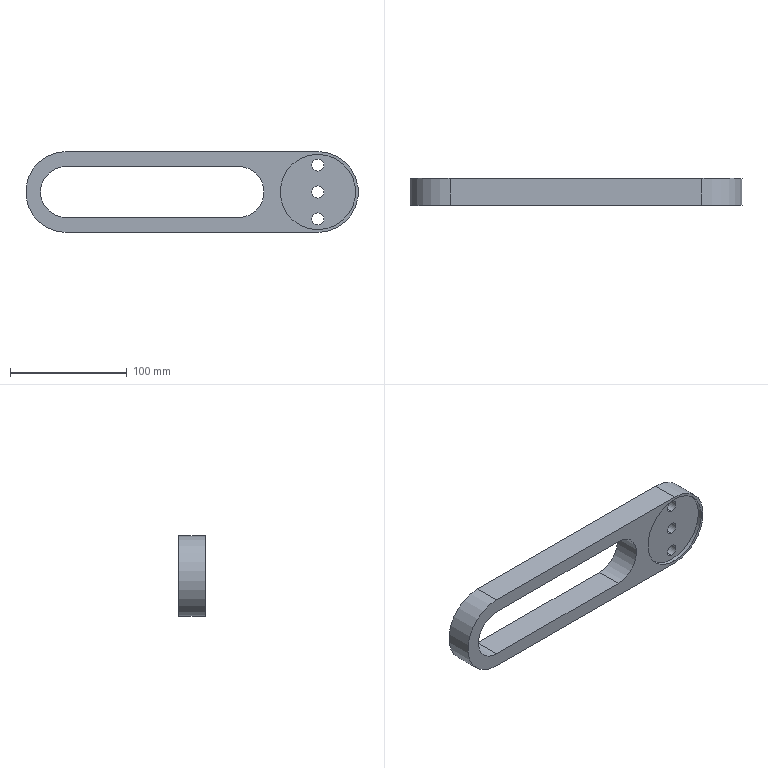Part | SolidWorks | features BaseBody 1 | 1 solid | 28 faces | box 285 x 23.077 x 69.231 mm | volume 225142 mm3 | cylinder 18 | plane 10 | commonest cylinder face diameters 10.385 x6 18.462 x6 43.846 x2 64.615 x2 69.231 x2
STEP:
#1=CARTESIAN_POINT('',(207.247,318.5,260.));
#2=VERTEX_POINT('',#1);
#3=CARTESIAN_POINT('',(207.247,318.5,278.462));
#4=VERTEX_POINT('',#3);
#5=CARTESIAN_POINT('',(207.247,318.5,269.231));
#6=DIRECTION('',(0.,1.,0.));
#7=DIRECTION('',(0.,0.,1.));
#8=AXIS2_PLACEMENT_3D('',#5,#6,#7);
#9=CIRCLE('',#8,9.231);
#10=EDGE_CURVE('',#2,#4,#9,.T.);
#11=ORIENTED_EDGE('',*,*,#10,.F.);
#12=CARTESIAN_POINT('',(207.247,329.115,260.));
#13=VERTEX_POINT('',#12);
#14=CARTESIAN_POINT('',(207.247,306.039,260.));
#15=DIRECTION('',(0.,1.,0.));
#16=VECTOR('',#15,1000.);
#17=LINE('',#14,#16);
#18=EDGE_CURVE('',#2,#13,#17,.T.);
#19=ORIENTED_EDGE('',*,*,#18,.T.);
#20=CARTESIAN_POINT('',(207.247,329.115,278.462));
#21=VERTEX_POINT('',#20);
#22=CARTESIAN_POINT('',(207.247,329.115,269.231));
#23=DIRECTION('',(0.,-1.,0.));
#24=DIRECTION('',(0.,0.,1.));
#25=AXIS2_PLACEMENT_3D('',#22,#23,#24);
#26=CIRCLE('',#25,9.231);
#27=EDGE_CURVE('',#21,#13,#26,.T.);
#28=ORIENTED_EDGE('',*,*,#27,.F.);
#29=CARTESIAN_POINT('',(207.247,306.039,278.462));
#30=DIRECTION('',(0.,1.,0.));
#31=VECTOR('',#30,1000.);
#32=LINE('',#29,#31);
#33=EDGE_CURVE('',#4,#21,#32,.T.);
#34=ORIENTED_EDGE('',*,*,#33,.F.);
#35=EDGE_LOOP('',(#11,#19,#28,#34));
#36=FACE_OUTER_BOUND('',#35,.T.);
#37=CARTESIAN_POINT('',(207.247,306.039,269.231));
#38=DIRECTION('',(0.,1.,0.));
#39=DIRECTION('',(0.,0.,1.));
#40=AXIS2_PLACEMENT_3D('',#37,#38,#39);
#41=CYLINDRICAL_SURFACE('',#40,9.231);
#42=ADVANCED_FACE('',(#36),#41,.F.);
#43=CARTESIAN_POINT('',(207.247,318.5,236.923));
#44=VERTEX_POINT('',#43);
#45=CARTESIAN_POINT('',(207.247,318.5,255.385));
#46=VERTEX_POINT('',#45);
#47=CARTESIAN_POINT('',(207.247,318.5,246.154));
#48=DIRECTION('',(0.,1.,0.));
#49=DIRECTION('',(0.,0.,1.));
#50=AXIS2_PLACEMENT_3D('',#47,#48,#49);
#51=CIRCLE('',#50,9.231);
#52=EDGE_CURVE('',#44,#46,#51,.T.);
#53=ORIENTED_EDGE('',*,*,#52,.F.);
#54=CARTESIAN_POINT('',(207.247,329.115,236.923));
#55=VERTEX_POINT('',#54);
#56=CARTESIAN_POINT('',(207.247,306.039,236.923));
#57=DIRECTION('',(0.,1.,0.));
#58=VECTOR('',#57,1000.);
#59=LINE('',#56,#58);
#60=EDGE_CURVE('',#44,#55,#59,.T.);
#61=ORIENTED_EDGE('',*,*,#60,.T.);
#62=CARTESIAN_POINT('',(207.247,329.115,255.385));
#63=VERTEX_POINT('',#62);
#64=CARTESIAN_POINT('',(207.247,329.115,246.154));
#65=DIRECTION('',(0.,-1.,0.));
#66=DIRECTION('',(0.,0.,1.));
#67=AXIS2_PLACEMENT_3D('',#64,#65,#66);
#68=CIRCLE('',#67,9.231);
#69=EDGE_CURVE('',#63,#55,#68,.T.);
#70=ORIENTED_EDGE('',*,*,#69,.F.);
#71=CARTESIAN_POINT('',(207.247,306.039,255.385));
#72=DIRECTION('',(0.,1.,0.));
#73=VECTOR('',#72,1000.);
#74=LINE('',#71,#73);
#75=EDGE_CURVE('',#46,#63,#74,.T.);
#76=ORIENTED_EDGE('',*,*,#75,.F.);
#77=EDGE_LOOP('',(#53,#61,#70,#76));
#78=FACE_OUTER_BOUND('',#77,.T.);
#79=CARTESIAN_POINT('',(207.247,306.039,246.154));
#80=DIRECTION('',(0.,1.,0.));
#81=DIRECTION('',(0.,0.,1.));
#82=AXIS2_PLACEMENT_3D('',#79,#80,#81);
#83=CYLINDRICAL_SURFACE('',#82,9.231);
#84=ADVANCED_FACE('',(#78),#83,.F.);
#85=CARTESIAN_POINT('',(207.247,318.5,213.846));
#86=VERTEX_POINT('',#85);
#87=CARTESIAN_POINT('',(207.247,318.5,232.308));
#88=VERTEX_POINT('',#87);
#89=CARTESIAN_POINT('',(207.247,318.5,223.077));
#90=DIRECTION('',(0.,1.,0.));
#91=DIRECTION('',(0.,0.,1.));
#92=AXIS2_PLACEMENT_3D('',#89,#90,#91);
#93=CIRCLE('',#92,9.231);
#94=EDGE_CURVE('',#86,#88,#93,.T.);
#95=ORIENTED_EDGE('',*,*,#94,.F.);
#96=CARTESIAN_POINT('',(207.247,329.115,213.846));
#97=VERTEX_POINT('',#96);
#98=CARTESIAN_POINT('',(207.247,306.039,213.846));
#99=DIRECTION('',(0.,1.,0.));
#100=VECTOR('',#99,1000.);
#101=LINE('',#98,#100);
#102=EDGE_CURVE('',#86,#97,#101,.T.);
#103=ORIENTED_EDGE('',*,*,#102,.T.);
#104=CARTESIAN_POINT('',(207.247,329.115,232.308));
#105=VERTEX_POINT('',#104);
#106=CARTESIAN_POINT('',(207.247,329.115,223.077));
#107=DIRECTION('',(0.,-1.,0.));
#108=DIRECTION('',(0.,0.,1.));
#109=AXIS2_PLACEMENT_3D('',#106,#107,#108);
#110=CIRCLE('',#109,9.231);
#111=EDGE_CURVE('',#105,#97,#110,.T.);
#112=ORIENTED_EDGE('',*,*,#111,.F.);
#113=CARTESIAN_POINT('',(207.247,306.039,232.308));
#114=DIRECTION('',(0.,1.,0.));
#115=VECTOR('',#114,1000.);
#116=LINE('',#113,#115);
#117=EDGE_CURVE('',#88,#105,#116,.T.);
#118=ORIENTED_EDGE('',*,*,#117,.F.);
#119=EDGE_LOOP('',(#95,#103,#112,#118));
#120=FACE_OUTER_BOUND('',#119,.T.);
#121=CARTESIAN_POINT('',(207.247,306.039,223.077));
#122=DIRECTION('',(0.,1.,0.));
#123=DIRECTION('',(0.,0.,1.));
#124=AXIS2_PLACEMENT_3D('',#121,#122,#123);
#125=CYLINDRICAL_SURFACE('',#124,9.231);
#126=ADVANCED_FACE('',(#120),#125,.F.);
#127=CARTESIAN_POINT('',(207.247,309.5,264.038));
#128=VERTEX_POINT('',#127);
#129=CARTESIAN_POINT('',(207.247,309.5,274.423));
#130=VERTEX_POINT('',#129);
#131=CARTESIAN_POINT('',(207.247,309.5,269.231));
#132=DIRECTION('',(0.,1.,0.));
#133=DIRECTION('',(0.,0.,1.));
#134=AXIS2_PLACEMENT_3D('',#131,#132,#133);
#135=CIRCLE('',#134,5.192);
#136=EDGE_CURVE('',#128,#130,#135,.T.);
#137=ORIENTED_EDGE('',*,*,#136,.F.);
#138=CARTESIAN_POINT('',(207.247,318.5,264.038));
#139=VERTEX_POINT('',#138);
#140=CARTESIAN_POINT('',(207.247,306.039,264.038));
#141=DIRECTION('',(0.,1.,0.));
#142=VECTOR('',#141,1000.);
#143=LINE('',#140,#142);
#144=EDGE_CURVE('',#128,#139,#143,.T.);
#145=ORIENTED_EDGE('',*,*,#144,.T.);
#146=CARTESIAN_POINT('',(207.247,318.5,274.423));
#147=VERTEX_POINT('',#146);
#148=CARTESIAN_POINT('',(207.247,318.5,269.231));
#149=DIRECTION('',(0.,-1.,0.));
#150=DIRECTION('',(0.,0.,1.));
#151=AXIS2_PLACEMENT_3D('',#148,#149,#150);
#152=CIRCLE('',#151,5.192);
#153=EDGE_CURVE('',#147,#139,#152,.T.);
#154=ORIENTED_EDGE('',*,*,#153,.F.);
#155=CARTESIAN_POINT('',(207.247,306.039,274.423));
#156=DIRECTION('',(0.,1.,0.));
#157=VECTOR('',#156,1000.);
#158=LINE('',#155,#157);
#159=EDGE_CURVE('',#130,#147,#158,.T.);
#160=ORIENTED_EDGE('',*,*,#159,.F.);
#161=EDGE_LOOP('',(#137,#145,#154,#160));
#162=FACE_OUTER_BOUND('',#161,.T.);
#163=CARTESIAN_POINT('',(207.247,306.039,269.231));
#164=DIRECTION('',(0.,1.,0.));
#165=DIRECTION('',(0.,0.,1.));
#166=AXIS2_PLACEMENT_3D('',#163,#164,#165);
#167=CYLINDRICAL_SURFACE('',#166,5.192);
#168=ADVANCED_FACE('',(#162),#167,.F.);
#169=CARTESIAN_POINT('',(207.247,309.5,240.962));
#170=VERTEX_POINT('',#169);
#171=CARTESIAN_POINT('',(207.247,309.5,251.346));
#172=VERTEX_POINT('',#171);
#173=CARTESIAN_POINT('',(207.247,309.5,246.154));
#174=DIRECTION('',(0.,1.,0.));
#175=DIRECTION('',(0.,0.,1.));
#176=AXIS2_PLACEMENT_3D('',#173,#174,#175);
#177=CIRCLE('',#176,5.192);
#178=EDGE_CURVE('',#170,#172,#177,.T.);
#179=ORIENTED_EDGE('',*,*,#178,.F.);
#180=CARTESIAN_POINT('',(207.247,318.5,240.962));
#181=VERTEX_POINT('',#180);
#182=CARTESIAN_POINT('',(207.247,306.039,240.962));
#183=DIRECTION('',(0.,1.,0.));
#184=VECTOR('',#183,1000.);
#185=LINE('',#182,#184);
#186=EDGE_CURVE('',#170,#181,#185,.T.);
#187=ORIENTED_EDGE('',*,*,#186,.T.);
#188=CARTESIAN_POINT('',(207.247,318.5,251.346));
#189=VERTEX_POINT('',#188);
#190=CARTESIAN_POINT('',(207.247,318.5,246.154));
#191=DIRECTION('',(0.,-1.,0.));
#192=DIRECTION('',(0.,0.,1.));
#193=AXIS2_PLACEMENT_3D('',#190,#191,#192);
#194=CIRCLE('',#193,5.192);
#195=EDGE_CURVE('',#189,#181,#194,.T.);
#196=ORIENTED_EDGE('',*,*,#195,.F.);
#197=CARTESIAN_POINT('',(207.247,306.039,251.346));
#198=DIRECTION('',(0.,1.,0.));
#199=VECTOR('',#198,1000.);
#200=LINE('',#197,#199);
#201=EDGE_CURVE('',#172,#189,#200,.T.);
#202=ORIENTED_EDGE('',*,*,#201,.F.);
#203=EDGE_LOOP('',(#179,#187,#196,#202));
#204=FACE_OUTER_BOUND('',#203,.T.);
#205=CARTESIAN_POINT('',(207.247,306.039,246.154));
#206=DIRECTION('',(0.,1.,0.));
#207=DIRECTION('',(0.,0.,1.));
#208=AXIS2_PLACEMENT_3D('',#205,#206,#207);
#209=CYLINDRICAL_SURFACE('',#208,5.192);
#210=ADVANCED_FACE('',(#204),#209,.F.);
#211=CARTESIAN_POINT('',(207.247,306.039,278.462));
#212=VERTEX_POINT('',#211);
#213=CARTESIAN_POINT('',(207.247,306.039,213.846));
#214=VERTEX_POINT('',#213);
#215=CARTESIAN_POINT('',(207.247,306.039,246.154));
#216=DIRECTION('',(0.,-1.,0.));
#217=DIRECTION('',(0.,0.,1.));
#218=AXIS2_PLACEMENT_3D('',#215,#216,#217);
#219=CIRCLE('',#218,32.308);
#220=EDGE_CURVE('',#212,#214,#219,.T.);
#221=ORIENTED_EDGE('',*,*,#220,.T.);
#222=CARTESIAN_POINT('',(207.247,309.5,213.846));
#223=VERTEX_POINT('',#222);
#224=CARTESIAN_POINT('',(207.247,306.039,213.846));
#225=DIRECTION('',(0.,1.,0.));
#226=VECTOR('',#225,1000.);
#227=LINE('',#224,#226);
#228=EDGE_CURVE('',#214,#223,#227,.T.);
#229=ORIENTED_EDGE('',*,*,#228,.T.);
#230=CARTESIAN_POINT('',(207.247,309.5,278.462));
#231=VERTEX_POINT('',#230);
#232=CARTESIAN_POINT('',(207.247,309.5,246.154));
#233=DIRECTION('',(0.,-1.,0.));
#234=DIRECTION('',(0.,0.,1.));
#235=AXIS2_PLACEMENT_3D('',#232,#233,#234);
#236=CIRCLE('',#235,32.308);
#237=EDGE_CURVE('',#231,#223,#236,.T.);
#238=ORIENTED_EDGE('',*,*,#237,.F.);
#239=CARTESIAN_POINT('',(207.247,306.039,278.462));
#240=DIRECTION('',(0.,1.,0.));
#241=VECTOR('',#240,1000.);
#242=LINE('',#239,#241);
#243=EDGE_CURVE('',#212,#231,#242,.T.);
#244=ORIENTED_EDGE('',*,*,#243,.F.);
#245=EDGE_LOOP('',(#221,#229,#238,#244));
#246=FACE_OUTER_BOUND('',#245,.T.);
#247=CARTESIAN_POINT('',(207.247,306.039,246.154));
#248=DIRECTION('',(0.,1.,0.));
#249=DIRECTION('',(0.,0.,1.));
#250=AXIS2_PLACEMENT_3D('',#247,#248,#249);
#251=CYLINDRICAL_SURFACE('',#250,32.308);
#252=ADVANCED_FACE('',(#246),#251,.F.);
#253=CARTESIAN_POINT('',(207.247,309.5,217.885));
#254=VERTEX_POINT('',#253);
#255=CARTESIAN_POINT('',(207.247,309.5,228.269));
#256=VERTEX_POINT('',#255);
#257=CARTESIAN_POINT('',(207.247,309.5,223.077));
#258=DIRECTION('',(0.,1.,0.));
#259=DIRECTION('',(0.,0.,1.));
#260=AXIS2_PLACEMENT_3D('',#257,#258,#259);
#261=CIRCLE('',#260,5.192);
#262=EDGE_CURVE('',#254,#256,#261,.T.);
#263=ORIENTED_EDGE('',*,*,#262,.F.);
#264=CARTESIAN_POINT('',(207.247,318.5,217.885));
#265=VERTEX_POINT('',#264);
#266=CARTESIAN_POINT('',(207.247,306.039,217.885));
#267=DIRECTION('',(0.,1.,0.));
#268=VECTOR('',#267,1000.);
#269=LINE('',#266,#268);
#270=EDGE_CURVE('',#254,#265,#269,.T.);
#271=ORIENTED_EDGE('',*,*,#270,.T.);
#272=CARTESIAN_POINT('',(207.247,318.5,228.269));
#273=VERTEX_POINT('',#272);
#274=CARTESIAN_POINT('',(207.247,318.5,223.077));
#275=DIRECTION('',(0.,-1.,0.));
#276=DIRECTION('',(0.,0.,1.));
#277=AXIS2_PLACEMENT_3D('',#274,#275,#276);
#278=CIRCLE('',#277,5.192);
#279=EDGE_CURVE('',#273,#265,#278,.T.);
#280=ORIENTED_EDGE('',*,*,#279,.F.);
#281=CARTESIAN_POINT('',(207.247,306.039,228.269));
#282=DIRECTION('',(0.,1.,0.));
#283=VECTOR('',#282,1000.);
#284=LINE('',#281,#283);
#285=EDGE_CURVE('',#256,#273,#284,.T.);
#286=ORIENTED_EDGE('',*,*,#285,.F.);
#287=EDGE_LOOP('',(#263,#271,#280,#286));
#288=FACE_OUTER_BOUND('',#287,.T.);
#289=CARTESIAN_POINT('',(207.247,306.039,223.077));
#290=DIRECTION('',(0.,1.,0.));
#291=DIRECTION('',(0.,0.,1.));
#292=AXIS2_PLACEMENT_3D('',#289,#290,#291);
#293=CYLINDRICAL_SURFACE('',#292,5.192);
#294=ADVANCED_FACE('',(#288),#293,.F.);
#295=ORIENTED_EDGE('',*,*,#27,.T.);
#296=CARTESIAN_POINT('',(207.247,329.115,269.231));
#297=DIRECTION('',(0.,-1.,0.));
#298=DIRECTION('',(0.,0.,1.));
#299=AXIS2_PLACEMENT_3D('',#296,#297,#298);
#300=CIRCLE('',#299,9.231);
#301=EDGE_CURVE('',#13,#21,#300,.T.);
#302=ORIENTED_EDGE('',*,*,#301,.T.);
#303=EDGE_LOOP('',(#295,#302));
#304=FACE_BOUND('',#303,.T.);
#305=ORIENTED_EDGE('',*,*,#69,.T.);
#306=CARTESIAN_POINT('',(207.247,329.115,246.154));
#307=DIRECTION('',(0.,-1.,0.));
#308=DIRECTION('',(0.,0.,1.));
#309=AXIS2_PLACEMENT_3D('',#306,#307,#308);
#310=CIRCLE('',#309,9.231);
#311=EDGE_CURVE('',#55,#63,#310,.T.);
#312=ORIENTED_EDGE('',*,*,#311,.T.);
#313=EDGE_LOOP('',(#305,#312));
#314=FACE_BOUND('',#313,.T.);
#315=CARTESIAN_POINT('',(-8.523,329.115,268.077));
#316=VERTEX_POINT('',#315);
#317=CARTESIAN_POINT('',(-8.523,329.115,224.231));
#318=VERTEX_POINT('',#317);
#319=CARTESIAN_POINT('',(-8.523,329.115,246.154));
#320=DIRECTION('',(0.,-1.,0.));
#321=DIRECTION('',(0.,0.,1.));
#322=AXIS2_PLACEMENT_3D('',#319,#320,#321);
#323=CIRCLE('',#322,21.923);
#324=EDGE_CURVE('',#316,#318,#323,.T.);
#325=ORIENTED_EDGE('',*,*,#324,.T.);
#326=CARTESIAN_POINT('',(139.17,329.115,224.231));
#327=VERTEX_POINT('',#326);
#328=CARTESIAN_POINT('',(207.247,329.115,224.231));
#329=DIRECTION('',(1.,0.,0.));
#330=VECTOR('',#329,1000.);
#331=LINE('',#328,#330);
#332=EDGE_CURVE('',#318,#327,#331,.T.);
#333=ORIENTED_EDGE('',*,*,#332,.T.);
#334=CARTESIAN_POINT('',(139.17,329.115,268.077));
#335=VERTEX_POINT('',#334);
#336=CARTESIAN_POINT('',(139.17,329.115,246.154));
#337=DIRECTION('',(0.,-1.,0.));
#338=DIRECTION('',(0.,0.,1.));
#339=AXIS2_PLACEMENT_3D('',#336,#337,#338);
#340=CIRCLE('',#339,21.923);
#341=EDGE_CURVE('',#327,#335,#340,.T.);
#342=ORIENTED_EDGE('',*,*,#341,.T.);
#343=CARTESIAN_POINT('',(207.247,329.115,268.077));
#344=DIRECTION('',(-1.,0.,0.));
#345=VECTOR('',#344,1000.);
#346=LINE('',#343,#345);
#347=EDGE_CURVE('',#335,#316,#346,.T.);
#348=ORIENTED_EDGE('',*,*,#347,.T.);
#349=EDGE_LOOP('',(#325,#333,#342,#348));
#350=FACE_BOUND('',#349,.T.);
#351=ORIENTED_EDGE('',*,*,#111,.T.);
#352=CARTESIAN_POINT('',(207.247,329.115,223.077));
#353=DIRECTION('',(0.,-1.,0.));
#354=DIRECTION('',(0.,0.,1.));
#355=AXIS2_PLACEMENT_3D('',#352,#353,#354);
#356=CIRCLE('',#355,9.231);
#357=EDGE_CURVE('',#97,#105,#356,.T.);
#358=ORIENTED_EDGE('',*,*,#357,.T.);
#359=EDGE_LOOP('',(#351,#358));
#360=FACE_BOUND('',#359,.T.);
#361=CARTESIAN_POINT('',(207.247,329.115,280.769));
#362=VERTEX_POINT('',#361);
#363=CARTESIAN_POINT('',(207.247,329.115,211.538));
#364=VERTEX_POINT('',#363);
#365=CARTESIAN_POINT('',(207.247,329.115,246.154));
#366=DIRECTION('',(0.,1.,0.));
#367=DIRECTION('',(0.,0.,1.));
#368=AXIS2_PLACEMENT_3D('',#365,#366,#367);
#369=CIRCLE('',#368,34.615);
#370=EDGE_CURVE('',#362,#364,#369,.T.);
#371=ORIENTED_EDGE('',*,*,#370,.T.);
#372=CARTESIAN_POINT('',(-8.523,329.115,211.538));
#373=VERTEX_POINT('',#372);
#374=CARTESIAN_POINT('',(207.247,329.115,211.538));
#375=DIRECTION('',(-1.,0.,0.));
#376=VECTOR('',#375,1000.);
#377=LINE('',#374,#376);
#378=EDGE_CURVE('',#364,#373,#377,.T.);
#379=ORIENTED_EDGE('',*,*,#378,.T.);
#380=CARTESIAN_POINT('',(-8.523,329.115,280.769));
#381=VERTEX_POINT('',#380);
#382=CARTESIAN_POINT('',(-8.523,329.115,246.154));
#383=DIRECTION('',(0.,1.,0.));
#384=DIRECTION('',(0.,0.,1.));
#385=AXIS2_PLACEMENT_3D('',#382,#383,#384);
#386=CIRCLE('',#385,34.615);
#387=EDGE_CURVE('',#373,#381,#386,.T.);
#388=ORIENTED_EDGE('',*,*,#387,.T.);
#389=CARTESIAN_POINT('',(207.247,329.115,280.769));
#390=DIRECTION('',(1.,0.,0.));
#391=VECTOR('',#390,1000.);
#392=LINE('',#389,#391);
#393=EDGE_CURVE('',#381,#362,#392,.T.);
#394=ORIENTED_EDGE('',*,*,#393,.T.);
#395=EDGE_LOOP('',(#371,#379,#388,#394));
#396=FACE_OUTER_BOUND('',#395,.T.);
#397=CARTESIAN_POINT('',(207.247,329.115,246.154));
#398=DIRECTION('',(0.,1.,0.));
#399=DIRECTION('',(0.,0.,1.));
#400=AXIS2_PLACEMENT_3D('',#397,#398,#399);
#401=PLANE('',#400);
#402=ADVANCED_FACE('',(#304,#314,#350,#360,#396),#401,.T.);
#403=ORIENTED_EDGE('',*,*,#18,.F.);
#404=CARTESIAN_POINT('',(207.247,318.5,269.231));
#405=DIRECTION('',(0.,1.,0.));
#406=DIRECTION('',(0.,0.,1.));
#407=AXIS2_PLACEMENT_3D('',#404,#405,#406);
#408=CIRCLE('',#407,9.231);
#409=EDGE_CURVE('',#4,#2,#408,.T.);
#410=ORIENTED_EDGE('',*,*,#409,.F.);
#411=ORIENTED_EDGE('',*,*,#33,.T.);
#412=ORIENTED_EDGE('',*,*,#301,.F.);
#413=EDGE_LOOP('',(#403,#410,#411,#412));
#414=FACE_OUTER_BOUND('',#413,.T.);
#415=CARTESIAN_POINT('',(207.247,306.039,269.231));
#416=DIRECTION('',(0.,1.,0.));
#417=DIRECTION('',(0.,0.,1.));
#418=AXIS2_PLACEMENT_3D('',#415,#416,#417);
#419=CYLINDRICAL_SURFACE('',#418,9.231);
#420=ADVANCED_FACE('',(#414),#419,.F.);
#421=ORIENTED_EDGE('',*,*,#60,.F.);
#422=CARTESIAN_POINT('',(207.247,318.5,246.154));
#423=DIRECTION('',(0.,1.,0.));
#424=DIRECTION('',(0.,0.,1.));
#425=AXIS2_PLACEMENT_3D('',#422,#423,#424);
#426=CIRCLE('',#425,9.231);
#427=EDGE_CURVE('',#46,#44,#426,.T.);
#428=ORIENTED_EDGE('',*,*,#427,.F.);
#429=ORIENTED_EDGE('',*,*,#75,.T.);
#430=ORIENTED_EDGE('',*,*,#311,.F.);
#431=EDGE_LOOP('',(#421,#428,#429,#430));
#432=FACE_OUTER_BOUND('',#431,.T.);
#433=CARTESIAN_POINT('',(207.247,306.039,246.154));
#434=DIRECTION('',(0.,1.,0.));
#435=DIRECTION('',(0.,0.,1.));
#436=AXIS2_PLACEMENT_3D('',#433,#434,#435);
#437=CYLINDRICAL_SURFACE('',#436,9.231);
#438=ADVANCED_FACE('',(#432),#437,.F.);
#439=CARTESIAN_POINT('',(139.17,306.039,224.231));
#440=VERTEX_POINT('',#439);
#441=CARTESIAN_POINT('',(139.17,329.115,224.231));
#442=DIRECTION('',(0.,1.,0.));
#443=VECTOR('',#442,1000.);
#444=LINE('',#441,#443);
#445=EDGE_CURVE('',#440,#327,#444,.T.);
#446=ORIENTED_EDGE('',*,*,#445,.T.);
#447=ORIENTED_EDGE('',*,*,#332,.F.);
#448=CARTESIAN_POINT('',(-8.523,306.039,224.231));
#449=VERTEX_POINT('',#448);
#450=CARTESIAN_POINT('',(-8.523,329.115,224.231));
#451=DIRECTION('',(0.,-1.,0.));
#452=VECTOR('',#451,1000.);
#453=LINE('',#450,#452);
#454=EDGE_CURVE('',#318,#449,#453,.T.);
#455=ORIENTED_EDGE('',*,*,#454,.T.);
#456=CARTESIAN_POINT('',(139.17,306.039,224.231));
#457=DIRECTION('',(1.,0.,0.));
#458=VECTOR('',#457,1000.);
#459=LINE('',#456,#458);
#460=EDGE_CURVE('',#449,#440,#459,.T.);
#461=ORIENTED_EDGE('',*,*,#460,.T.);
#462=EDGE_LOOP('',(#446,#447,#455,#461));
#463=FACE_OUTER_BOUND('',#462,.T.);
#464=CARTESIAN_POINT('',(139.17,329.115,224.231));
#465=DIRECTION('',(0.,0.,1.));
#466=DIRECTION('',(1.,0.,0.));
#467=AXIS2_PLACEMENT_3D('',#464,#465,#466);
#468=PLANE('',#467);
#469=ADVANCED_FACE('',(#463),#468,.T.);
#470=CARTESIAN_POINT('',(-8.523,306.039,268.077));
#471=VERTEX_POINT('',#470);
#472=CARTESIAN_POINT('',(-8.523,329.115,268.077));
#473=DIRECTION('',(0.,1.,0.));
#474=VECTOR('',#473,1000.);
#475=LINE('',#472,#474);
#476=EDGE_CURVE('',#471,#316,#475,.T.);
#477=ORIENTED_EDGE('',*,*,#476,.F.);
#478=CARTESIAN_POINT('',(-8.523,306.039,246.154));
#479=DIRECTION('',(0.,1.,0.));
#480=DIRECTION('',(0.,0.,1.));
#481=AXIS2_PLACEMENT_3D('',#478,#479,#480);
#482=CIRCLE('',#481,21.923);
#483=EDGE_CURVE('',#449,#471,#482,.T.);
#484=ORIENTED_EDGE('',*,*,#483,.F.);
#485=ORIENTED_EDGE('',*,*,#454,.F.);
#486=ORIENTED_EDGE('',*,*,#324,.F.);
#487=EDGE_LOOP('',(#477,#484,#485,#486));
#488=FACE_OUTER_BOUND('',#487,.T.);
#489=CARTESIAN_POINT('',(-8.523,329.115,246.154));
#490=DIRECTION('',(0.,1.,0.));
#491=DIRECTION('',(0.,0.,1.));
#492=AXIS2_PLACEMENT_3D('',#489,#490,#491);
#493=CYLINDRICAL_SURFACE('',#492,21.923);
#494=ADVANCED_FACE('',(#488),#493,.F.);
#495=ORIENTED_EDGE('',*,*,#476,.T.);
#496=ORIENTED_EDGE('',*,*,#347,.F.);
#497=CARTESIAN_POINT('',(139.17,306.039,268.077));
#498=VERTEX_POINT('',#497);
#499=CARTESIAN_POINT('',(139.17,329.115,268.077));
#500=DIRECTION('',(0.,-1.,0.));
#501=VECTOR('',#500,1000.);
#502=LINE('',#499,#501);
#503=EDGE_CURVE('',#335,#498,#502,.T.);
#504=ORIENTED_EDGE('',*,*,#503,.T.);
#505=CARTESIAN_POINT('',(-8.523,306.039,268.077));
#506=DIRECTION('',(-1.,0.,0.));
#507=VECTOR('',#506,1000.);
#508=LINE('',#505,#507);
#509=EDGE_CURVE('',#498,#471,#508,.T.);
#510=ORIENTED_EDGE('',*,*,#509,.T.);
#511=EDGE_LOOP('',(#495,#496,#504,#510));
#512=FACE_OUTER_BOUND('',#511,.T.);
#513=CARTESIAN_POINT('',(-8.523,329.115,268.077));
#514=DIRECTION('',(0.,0.,-1.));
#515=DIRECTION('',(-1.,0.,0.));
#516=AXIS2_PLACEMENT_3D('',#513,#514,#515);
#517=PLANE('',#516);
#518=ADVANCED_FACE('',(#512),#517,.T.);
#519=ORIENTED_EDGE('',*,*,#445,.F.);
#520=CARTESIAN_POINT('',(139.17,306.039,246.154));
#521=DIRECTION('',(0.,1.,0.));
#522=DIRECTION('',(0.,0.,1.));
#523=AXIS2_PLACEMENT_3D('',#520,#521,#522);
#524=CIRCLE('',#523,21.923);
#525=EDGE_CURVE('',#498,#440,#524,.T.);
#526=ORIENTED_EDGE('',*,*,#525,.F.);
#527=ORIENTED_EDGE('',*,*,#503,.F.);
#528=ORIENTED_EDGE('',*,*,#341,.F.);
#529=EDGE_LOOP('',(#519,#526,#527,#528));
#530=FACE_OUTER_BOUND('',#529,.T.);
#531=CARTESIAN_POINT('',(139.17,329.115,246.154));
#532=DIRECTION('',(0.,1.,0.));
#533=DIRECTION('',(0.,0.,1.));
#534=AXIS2_PLACEMENT_3D('',#531,#532,#533);
#535=CYLINDRICAL_SURFACE('',#534,21.923);
#536=ADVANCED_FACE('',(#530),#535,.F.);
#537=ORIENTED_EDGE('',*,*,#102,.F.);
#538=CARTESIAN_POINT('',(207.247,318.5,223.077));
#539=DIRECTION('',(0.,1.,0.));
#540=DIRECTION('',(0.,0.,1.));
#541=AXIS2_PLACEMENT_3D('',#538,#539,#540);
#542=CIRCLE('',#541,9.231);
#543=EDGE_CURVE('',#88,#86,#542,.T.);
#544=ORIENTED_EDGE('',*,*,#543,.F.);
#545=ORIENTED_EDGE('',*,*,#117,.T.);
#546=ORIENTED_EDGE('',*,*,#357,.F.);
#547=EDGE_LOOP('',(#537,#544,#545,#546));
#548=FACE_OUTER_BOUND('',#547,.T.);
#549=CARTESIAN_POINT('',(207.247,306.039,223.077));
#550=DIRECTION('',(0.,1.,0.));
#551=DIRECTION('',(0.,0.,1.));
#552=AXIS2_PLACEMENT_3D('',#549,#550,#551);
#553=CYLINDRICAL_SURFACE('',#552,9.231);
#554=ADVANCED_FACE('',(#548),#553,.F.);
#555=CARTESIAN_POINT('',(207.247,306.039,211.538));
#556=VERTEX_POINT('',#555);
#557=CARTESIAN_POINT('',(207.247,329.115,211.538));
#558=DIRECTION('',(0.,1.,0.));
#559=VECTOR('',#558,1000.);
#560=LINE('',#557,#559);
#561=EDGE_CURVE('',#556,#364,#560,.T.);
#562=ORIENTED_EDGE('',*,*,#561,.F.);
#563=CARTESIAN_POINT('',(-8.523,306.039,211.538));
#564=VERTEX_POINT('',#563);
#565=CARTESIAN_POINT('',(207.247,306.039,211.538));
#566=DIRECTION('',(1.,0.,0.));
#567=VECTOR('',#566,1000.);
#568=LINE('',#565,#567);
#569=EDGE_CURVE('',#564,#556,#568,.T.);
#570=ORIENTED_EDGE('',*,*,#569,.F.);
#571=CARTESIAN_POINT('',(-8.523,329.115,211.538));
#572=DIRECTION('',(0.,-1.,0.));
#573=VECTOR('',#572,1000.);
#574=LINE('',#571,#573);
#575=EDGE_CURVE('',#373,#564,#574,.T.);
#576=ORIENTED_EDGE('',*,*,#575,.F.);
#577=ORIENTED_EDGE('',*,*,#378,.F.);
#578=EDGE_LOOP('',(#562,#570,#576,#577));
#579=FACE_OUTER_BOUND('',#578,.T.);
#580=CARTESIAN_POINT('',(207.247,329.115,211.538));
#581=DIRECTION('',(0.,0.,1.));
#582=DIRECTION('',(1.,0.,0.));
#583=AXIS2_PLACEMENT_3D('',#580,#581,#582);
#584=PLANE('',#583);
#585=ADVANCED_FACE('',(#579),#584,.F.);
#586=ORIENTED_EDGE('',*,*,#561,.T.);
#587=ORIENTED_EDGE('',*,*,#370,.F.);
#588=CARTESIAN_POINT('',(207.247,306.039,280.769));
#589=VERTEX_POINT('',#588);
#590=CARTESIAN_POINT('',(207.247,329.115,280.769));
#591=DIRECTION('',(0.,-1.,0.));
#592=VECTOR('',#591,1000.);
#593=LINE('',#590,#592);
#594=EDGE_CURVE('',#362,#589,#593,.T.);
#595=ORIENTED_EDGE('',*,*,#594,.T.);
#596=CARTESIAN_POINT('',(207.247,306.039,246.154));
#597=DIRECTION('',(0.,1.,0.));
#598=DIRECTION('',(0.,0.,1.));
#599=AXIS2_PLACEMENT_3D('',#596,#597,#598);
#600=CIRCLE('',#599,34.615);
#601=EDGE_CURVE('',#589,#556,#600,.T.);
#602=ORIENTED_EDGE('',*,*,#601,.T.);
#603=EDGE_LOOP('',(#586,#587,#595,#602));
#604=FACE_OUTER_BOUND('',#603,.T.);
#605=CARTESIAN_POINT('',(207.247,329.115,246.154));
#606=DIRECTION('',(0.,1.,0.));
#607=DIRECTION('',(0.,0.,1.));
#608=AXIS2_PLACEMENT_3D('',#605,#606,#607);
#609=CYLINDRICAL_SURFACE('',#608,34.615);
#610=ADVANCED_FACE('',(#604),#609,.T.);
#611=CARTESIAN_POINT('',(-8.523,306.039,280.769));
#612=VERTEX_POINT('',#611);
#613=CARTESIAN_POINT('',(-8.523,329.115,280.769));
#614=DIRECTION('',(0.,1.,0.));
#615=VECTOR('',#614,1000.);
#616=LINE('',#613,#615);
#617=EDGE_CURVE('',#612,#381,#616,.T.);
#618=ORIENTED_EDGE('',*,*,#617,.F.);
#619=CARTESIAN_POINT('',(-8.523,306.039,280.769));
#620=DIRECTION('',(-1.,0.,0.));
#621=VECTOR('',#620,1000.);
#622=LINE('',#619,#621);
#623=EDGE_CURVE('',#589,#612,#622,.T.);
#624=ORIENTED_EDGE('',*,*,#623,.F.);
#625=ORIENTED_EDGE('',*,*,#594,.F.);
#626=ORIENTED_EDGE('',*,*,#393,.F.);
#627=EDGE_LOOP('',(#618,#624,#625,#626));
#628=FACE_OUTER_BOUND('',#627,.T.);
#629=CARTESIAN_POINT('',(-8.523,329.115,280.769));
#630=DIRECTION('',(0.,0.,-1.));
#631=DIRECTION('',(-1.,0.,0.));
#632=AXIS2_PLACEMENT_3D('',#629,#630,#631);
#633=PLANE('',#632);
#634=ADVANCED_FACE('',(#628),#633,.F.);
#635=ORIENTED_EDGE('',*,*,#617,.T.);
#636=ORIENTED_EDGE('',*,*,#387,.F.);
#637=ORIENTED_EDGE('',*,*,#575,.T.);
#638=CARTESIAN_POINT('',(-8.523,306.039,246.154));
#639=DIRECTION('',(0.,1.,0.));
#640=DIRECTION('',(0.,0.,1.));
#641=AXIS2_PLACEMENT_3D('',#638,#639,#640);
#642=CIRCLE('',#641,34.615);
#643=EDGE_CURVE('',#564,#612,#642,.T.);
#644=ORIENTED_EDGE('',*,*,#643,.T.);
#645=EDGE_LOOP('',(#635,#636,#637,#644));
#646=FACE_OUTER_BOUND('',#645,.T.);
#647=CARTESIAN_POINT('',(-8.523,329.115,246.154));
#648=DIRECTION('',(0.,1.,0.));
#649=DIRECTION('',(0.,0.,1.));
#650=AXIS2_PLACEMENT_3D('',#647,#648,#649);
#651=CYLINDRICAL_SURFACE('',#650,34.615);
#652=ADVANCED_FACE('',(#646),#651,.T.);
#653=ORIENTED_EDGE('',*,*,#153,.T.);
#654=CARTESIAN_POINT('',(207.247,318.5,269.231));
#655=DIRECTION('',(0.,-1.,0.));
#656=DIRECTION('',(0.,0.,1.));
#657=AXIS2_PLACEMENT_3D('',#654,#655,#656);
#658=CIRCLE('',#657,5.192);
#659=EDGE_CURVE('',#139,#147,#658,.T.);
#660=ORIENTED_EDGE('',*,*,#659,.T.);
#661=EDGE_LOOP('',(#653,#660));
#662=FACE_BOUND('',#661,.T.);
#663=ORIENTED_EDGE('',*,*,#409,.T.);
#664=ORIENTED_EDGE('',*,*,#10,.T.);
#665=EDGE_LOOP('',(#663,#664));
#666=FACE_OUTER_BOUND('',#665,.T.);
#667=CARTESIAN_POINT('',(198.016,318.5,269.231));
#668=DIRECTION('',(0.,1.,0.));
#669=DIRECTION('',(0.,0.,1.));
#670=AXIS2_PLACEMENT_3D('',#667,#668,#669);
#671=PLANE('',#670);
#672=ADVANCED_FACE('',(#662,#666),#671,.T.);
#673=ORIENTED_EDGE('',*,*,#195,.T.);
#674=CARTESIAN_POINT('',(207.247,318.5,246.154));
#675=DIRECTION('',(0.,-1.,0.));
#676=DIRECTION('',(0.,0.,1.));
#677=AXIS2_PLACEMENT_3D('',#674,#675,#676);
#678=CIRCLE('',#677,5.192);
#679=EDGE_CURVE('',#181,#189,#678,.T.);
#680=ORIENTED_EDGE('',*,*,#679,.T.);
#681=EDGE_LOOP('',(#673,#680));
#682=FACE_BOUND('',#681,.T.);
#683=ORIENTED_EDGE('',*,*,#427,.T.);
#684=ORIENTED_EDGE('',*,*,#52,.T.);
#685=EDGE_LOOP('',(#683,#684));
#686=FACE_OUTER_BOUND('',#685,.T.);
#687=CARTESIAN_POINT('',(198.016,318.5,246.154));
#688=DIRECTION('',(0.,1.,0.));
#689=DIRECTION('',(0.,0.,1.));
#690=AXIS2_PLACEMENT_3D('',#687,#688,#689);
#691=PLANE('',#690);
#692=ADVANCED_FACE('',(#682,#686),#691,.T.);
#693=ORIENTED_EDGE('',*,*,#220,.F.);
#694=CARTESIAN_POINT('',(207.247,306.039,246.154));
#695=DIRECTION('',(0.,-1.,0.));
#696=DIRECTION('',(0.,0.,1.));
#697=AXIS2_PLACEMENT_3D('',#694,#695,#696);
#698=CIRCLE('',#697,32.308);
#699=EDGE_CURVE('',#214,#212,#698,.T.);
#700=ORIENTED_EDGE('',*,*,#699,.F.);
#701=EDGE_LOOP('',(#693,#700));
#702=FACE_BOUND('',#701,.T.);
#703=ORIENTED_EDGE('',*,*,#483,.T.);
#704=ORIENTED_EDGE('',*,*,#509,.F.);
#705=ORIENTED_EDGE('',*,*,#525,.T.);
#706=ORIENTED_EDGE('',*,*,#460,.F.);
#707=EDGE_LOOP('',(#703,#704,#705,#706));
#708=FACE_BOUND('',#707,.T.);
#709=ORIENTED_EDGE('',*,*,#601,.F.);
#710=ORIENTED_EDGE('',*,*,#623,.T.);
#711=ORIENTED_EDGE('',*,*,#643,.F.);
#712=ORIENTED_EDGE('',*,*,#569,.T.);
#713=EDGE_LOOP('',(#709,#710,#711,#712));
#714=FACE_OUTER_BOUND('',#713,.T.);
#715=CARTESIAN_POINT('',(207.247,306.039,246.154));
#716=DIRECTION('',(0.,1.,0.));
#717=DIRECTION('',(0.,0.,1.));
#718=AXIS2_PLACEMENT_3D('',#715,#716,#717);
#719=PLANE('',#718);
#720=ADVANCED_FACE('',(#702,#708,#714),#719,.F.);
#721=ORIENTED_EDGE('',*,*,#279,.T.);
#722=CARTESIAN_POINT('',(207.247,318.5,223.077));
#723=DIRECTION('',(0.,-1.,0.));
#724=DIRECTION('',(0.,0.,1.));
#725=AXIS2_PLACEMENT_3D('',#722,#723,#724);
#726=CIRCLE('',#725,5.192);
#727=EDGE_CURVE('',#265,#273,#726,.T.);
#728=ORIENTED_EDGE('',*,*,#727,.T.);
#729=EDGE_LOOP('',(#721,#728));
#730=FACE_BOUND('',#729,.T.);
#731=ORIENTED_EDGE('',*,*,#543,.T.);
#732=ORIENTED_EDGE('',*,*,#94,.T.);
#733=EDGE_LOOP('',(#731,#732));
#734=FACE_OUTER_BOUND('',#733,.T.);
#735=CARTESIAN_POINT('',(198.016,318.5,223.077));
#736=DIRECTION('',(0.,1.,0.));
#737=DIRECTION('',(0.,0.,1.));
#738=AXIS2_PLACEMENT_3D('',#735,#736,#737);
#739=PLANE('',#738);
#740=ADVANCED_FACE('',(#730,#734),#739,.T.);
#741=ORIENTED_EDGE('',*,*,#144,.F.);
#742=CARTESIAN_POINT('',(207.247,309.5,269.231));
#743=DIRECTION('',(0.,1.,0.));
#744=DIRECTION('',(0.,0.,1.));
#745=AXIS2_PLACEMENT_3D('',#742,#743,#744);
#746=CIRCLE('',#745,5.192);
#747=EDGE_CURVE('',#130,#128,#746,.T.);
#748=ORIENTED_EDGE('',*,*,#747,.F.);
#749=ORIENTED_EDGE('',*,*,#159,.T.);
#750=ORIENTED_EDGE('',*,*,#659,.F.);
#751=EDGE_LOOP('',(#741,#748,#749,#750));
#752=FACE_OUTER_BOUND('',#751,.T.);
#753=CARTESIAN_POINT('',(207.247,306.039,269.231));
#754=DIRECTION('',(0.,1.,0.));
#755=DIRECTION('',(0.,0.,1.));
#756=AXIS2_PLACEMENT_3D('',#753,#754,#755);
#757=CYLINDRICAL_SURFACE('',#756,5.192);
#758=ADVANCED_FACE('',(#752),#757,.F.);
#759=ORIENTED_EDGE('',*,*,#186,.F.);
#760=CARTESIAN_POINT('',(207.247,309.5,246.154));
#761=DIRECTION('',(0.,1.,0.));
#762=DIRECTION('',(0.,0.,1.));
#763=AXIS2_PLACEMENT_3D('',#760,#761,#762);
#764=CIRCLE('',#763,5.192);
#765=EDGE_CURVE('',#172,#170,#764,.T.);
#766=ORIENTED_EDGE('',*,*,#765,.F.);
#767=ORIENTED_EDGE('',*,*,#201,.T.);
#768=ORIENTED_EDGE('',*,*,#679,.F.);
#769=EDGE_LOOP('',(#759,#766,#767,#768));
#770=FACE_OUTER_BOUND('',#769,.T.);
#771=CARTESIAN_POINT('',(207.247,306.039,246.154));
#772=DIRECTION('',(0.,1.,0.));
#773=DIRECTION('',(0.,0.,1.));
#774=AXIS2_PLACEMENT_3D('',#771,#772,#773);
#775=CYLINDRICAL_SURFACE('',#774,5.192);
#776=ADVANCED_FACE('',(#770),#775,.F.);
#777=ORIENTED_EDGE('',*,*,#228,.F.);
#778=ORIENTED_EDGE('',*,*,#699,.T.);
#779=ORIENTED_EDGE('',*,*,#243,.T.);
#780=CARTESIAN_POINT('',(207.247,309.5,246.154));
#781=DIRECTION('',(0.,-1.,0.));
#782=DIRECTION('',(0.,0.,1.));
#783=AXIS2_PLACEMENT_3D('',#780,#781,#782);
#784=CIRCLE('',#783,32.308);
#785=EDGE_CURVE('',#223,#231,#784,.T.);
#786=ORIENTED_EDGE('',*,*,#785,.F.);
#787=EDGE_LOOP('',(#777,#778,#779,#786));
#788=FACE_OUTER_BOUND('',#787,.T.);
#789=CARTESIAN_POINT('',(207.247,306.039,246.154));
#790=DIRECTION('',(0.,1.,0.));
#791=DIRECTION('',(0.,0.,1.));
#792=AXIS2_PLACEMENT_3D('',#789,#790,#791);
#793=CYLINDRICAL_SURFACE('',#792,32.308);
#794=ADVANCED_FACE('',(#788),#793,.F.);
#795=ORIENTED_EDGE('',*,*,#270,.F.);
#796=CARTESIAN_POINT('',(207.247,309.5,223.077));
#797=DIRECTION('',(0.,1.,0.));
#798=DIRECTION('',(0.,0.,1.));
#799=AXIS2_PLACEMENT_3D('',#796,#797,#798);
#800=CIRCLE('',#799,5.192);
#801=EDGE_CURVE('',#256,#254,#800,.T.);
#802=ORIENTED_EDGE('',*,*,#801,.F.);
#803=ORIENTED_EDGE('',*,*,#285,.T.);
#804=ORIENTED_EDGE('',*,*,#727,.F.);
#805=EDGE_LOOP('',(#795,#802,#803,#804));
#806=FACE_OUTER_BOUND('',#805,.T.);
#807=CARTESIAN_POINT('',(207.247,306.039,223.077));
#808=DIRECTION('',(0.,1.,0.));
#809=DIRECTION('',(0.,0.,1.));
#810=AXIS2_PLACEMENT_3D('',#807,#808,#809);
#811=CYLINDRICAL_SURFACE('',#810,5.192);
#812=ADVANCED_FACE('',(#806),#811,.F.);
#813=ORIENTED_EDGE('',*,*,#765,.T.);
#814=ORIENTED_EDGE('',*,*,#178,.T.);
#815=EDGE_LOOP('',(#813,#814));
#816=FACE_BOUND('',#815,.T.);
#817=ORIENTED_EDGE('',*,*,#747,.T.);
#818=ORIENTED_EDGE('',*,*,#136,.T.);
#819=EDGE_LOOP('',(#817,#818));
#820=FACE_BOUND('',#819,.T.);
#821=ORIENTED_EDGE('',*,*,#801,.T.);
#822=ORIENTED_EDGE('',*,*,#262,.T.);
#823=EDGE_LOOP('',(#821,#822));
#824=FACE_BOUND('',#823,.T.);
#825=ORIENTED_EDGE('',*,*,#237,.T.);
#826=ORIENTED_EDGE('',*,*,#785,.T.);
#827=EDGE_LOOP('',(#825,#826));
#828=FACE_OUTER_BOUND('',#827,.T.);
#829=CARTESIAN_POINT('',(207.247,309.5,246.154));
#830=DIRECTION('',(0.,-1.,0.));
#831=DIRECTION('',(0.,0.,-1.));
#832=AXIS2_PLACEMENT_3D('',#829,#830,#831);
#833=PLANE('',#832);
#834=ADVANCED_FACE('',(#816,#820,#824,#828),#833,.T.);
#835=CLOSED_SHELL('',(#42,#84,#126,#168,#210,#252,#294,#402,#420,#438,#469,#494,#518,#536,#554,#585,#610,#634,#652,#672,#692,#720,#740,#758,#776,#794,#812,#834));
#836=MANIFOLD_SOLID_BREP('',#835);
#837=CARTESIAN_POINT('',(0.,0.,0.));
#838=DIRECTION('',(0.,0.,1.));
#839=DIRECTION('',(1.,0.,0.));
#840=AXIS2_PLACEMENT_3D('',#837,#838,#839);
#841=(LENGTH_UNIT()NAMED_UNIT(*)SI_UNIT(.MILLI.,.METRE.));
#842=UNCERTAINTY_MEASURE_WITH_UNIT(LENGTH_MEASURE(0.00001),#841,'','');
#843=(NAMED_UNIT(*)PLANE_ANGLE_UNIT()SI_UNIT($,.RADIAN.));
#844=(NAMED_UNIT(*)SI_UNIT($,.STERADIAN.)SOLID_ANGLE_UNIT());
#845=(GEOMETRIC_REPRESENTATION_CONTEXT(3)GLOBAL_UNCERTAINTY_ASSIGNED_CONTEXT((#842))GLOBAL_UNIT_ASSIGNED_CONTEXT((#841,#843,#844))REPRESENTATION_CONTEXT('',''));
#846=ADVANCED_BREP_SHAPE_REPRESENTATION('',(#836,#840),#845);